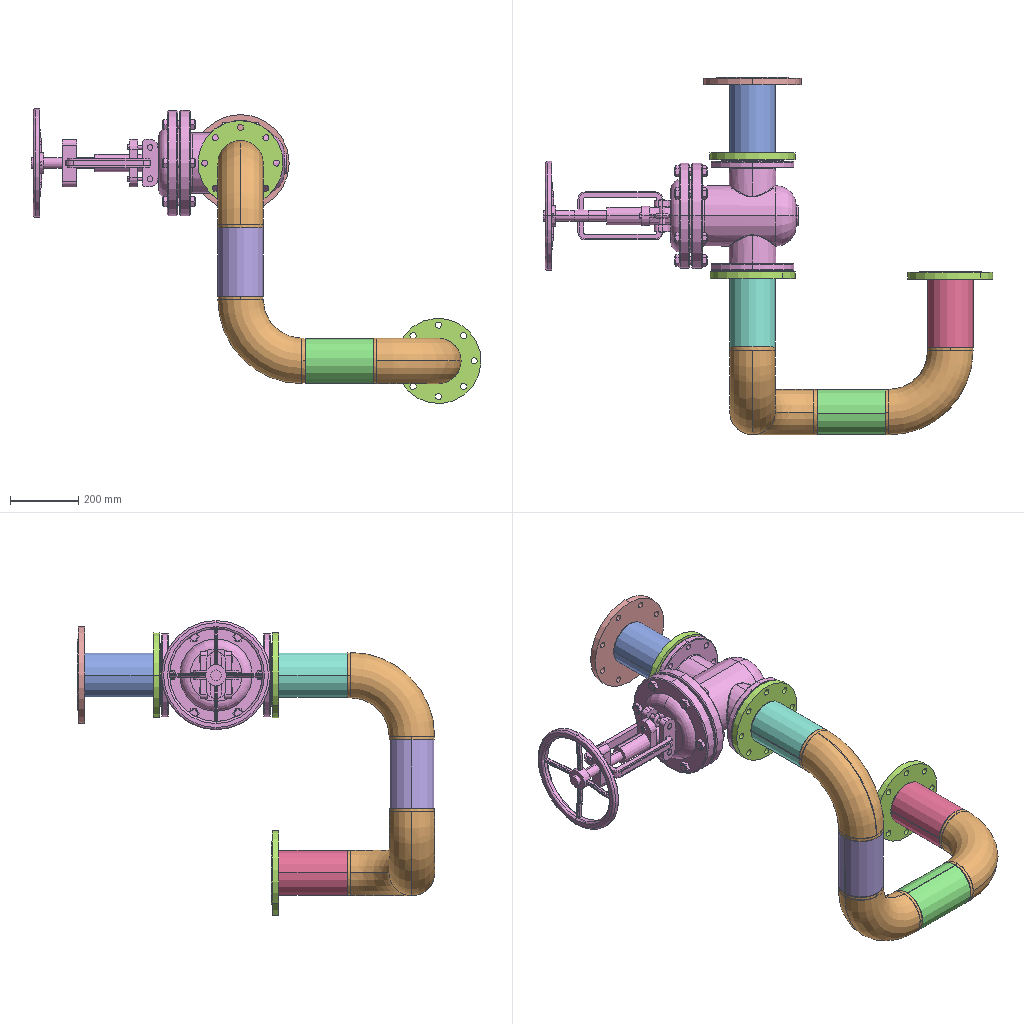Assembly | SolidWorks | 9 different items | 13 placed | box 1319 x 1048 x 865 mm
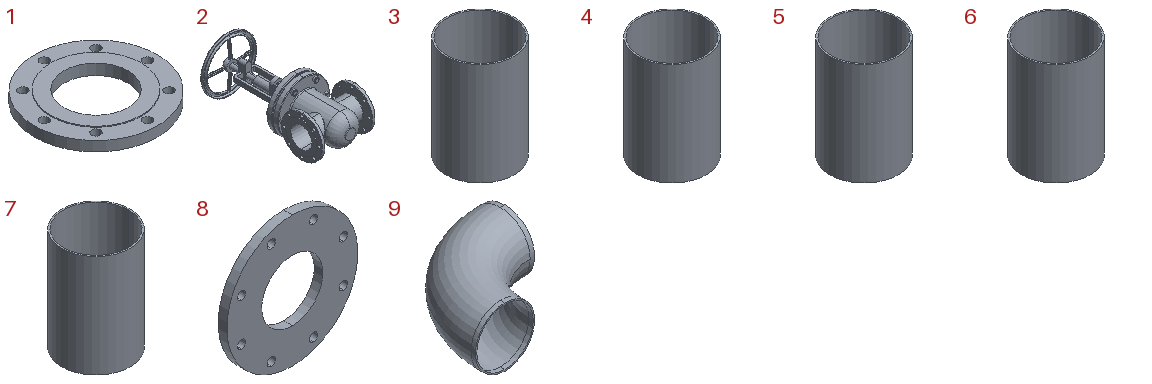Parts list (item | quantity | size | volume | features):
1 | x3 | 250 x 250 x 22 mm | 702203 mm3 | features Extrusion 1, ICE 1
2 | x1 | 325 x 747.833 x 320 mm | 15071073 mm3 | features BaseBody 1
3 | x1 | 133 x 133 x 200 mm | 245044 mm3 | features Extrusion 1
4 | x1 | 133 x 133 x 200 mm | 245044 mm3 | features Extrusion 1
5 | x1 | 133 x 133 x 200 mm | 245044 mm3 | features Extrusion 1
6 | x1 | 133 x 133 x 200 mm | 245044 mm3 | features Extrusion 1
7 | x1 | 133 x 133 x 200 mm | 245044 mm3 | features Extrusion 1
8 | x1 | 285 x 22 x 285 mm | 945255 mm3 | features ICE 2, CirPattern 1, Extrusion 1
9 | x3 | 256.5 x 256.5 x 133 mm | 370928 mm3 | features 3DProfileFeature 1, Shell 1, Sweep 1
Mates (type | each side: item.copy, entity, surface, feature):
Coincident | 8.1 face plane Boss-Extrude1 | 3.1 face plane Boss-Extrude1
Concentric | 8.1 face cylinder Boss-Extrude1 | 3.1 face cylinder Boss-Extrude1
Coincident | 3.1 face plane Boss-Extrude1 | 1.1 face plane Boss-Extrude1
Concentric | 3.1 face cylinder Boss-Extrude1 | 1.1 face cylinder Boss-Extrude1
Coincident | 8.1 plane | 1.1 plane
Coincident | 1.1 face plane Boss-Extrude2 | 2.1 face plane feature 17 (BaseBody) Input1
Concentric | 1.1 face cylinder Boss-Extrude1 | 2.1 face cylinder feature 17 (BaseBody) Input1 | 2 times
Coincident | 2.1 face plane feature 17 (BaseBody) Input1 | 1.2 face plane Boss-Extrude2
Concentric | 2.1 face cylinder feature 17 (BaseBody) Input1 | 1.2 face cylinder Boss-Extrude1 | 2 times
Coincident | 1.2 face plane Boss-Extrude1 | 4.1 face plane Boss-Extrude1
Concentric | 1.2 face cylinder Boss-Extrude1 | 4.1 face cylinder Boss-Extrude1
Coincident | 4.1 face plane Boss-Extrude1 | 9.1 face plane Sweep1
Concentric | 4.1 face cylinder Boss-Extrude1 | 9.1 face cylinder Sweep1
Coincident | 8.1 plane | 9.1 plane
Coincident | 9.1 face plane Sweep1 | 5.1 face plane Boss-Extrude1
Coincident | 9.1 edge | 5.1 face cylinder Boss-Extrude1
Coincident | 5.1 face plane Boss-Extrude1 | 9.2 face plane Sweep1
Concentric | 5.1 face cylinder Boss-Extrude1 | 9.2 face cylinder Sweep1
Coincident | 9.2 face plane Sweep1 | 6.1 face plane Boss-Extrude1
Concentric | 9.2 face cylinder Sweep1 | 6.1 face cylinder Boss-Extrude1
Coincident | 6.1 face plane Boss-Extrude1 | 9.3 face plane Sweep1
Concentric | 6.1 face cylinder Boss-Extrude1 | 9.3 face cylinder Sweep1
Coincident | 9.3 face plane Sweep1 | 7.1 face plane Boss-Extrude1
Concentric | 9.3 face cylinder Sweep1 | 7.1 face cylinder Boss-Extrude1
Coincident | 7.1 face plane Boss-Extrude1 | 1.3 face plane Boss-Extrude1
Concentric | 7.1 face cylinder Boss-Extrude1 | 1.3 face cylinder Boss-Extrude1
Parallel | 8.1 face plane Boss-Extrude1 | 1.3 face plane Boss-Extrude2